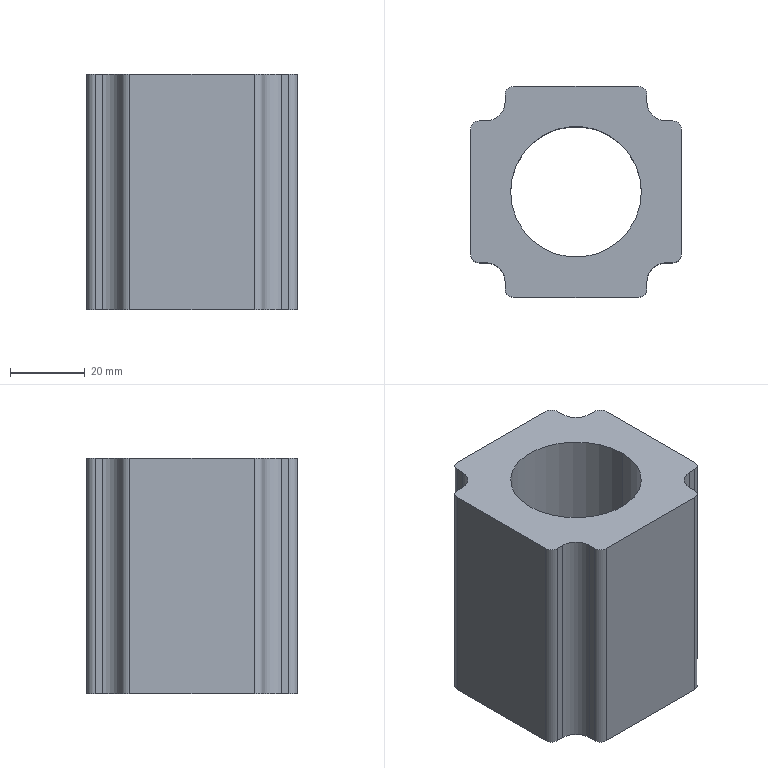Part | SolidWorks | features BaseBody 1 | 1 solid | 28 faces | box 56.4 x 56.4 x 63 mm | volume 119307 mm3 | cylinder 14 | plane 14 | commonest cylinder face diameters 4.6 x8 10 x4 34.98 x2
STEP:
#1=CARTESIAN_POINT('',(17.49,0.,-10.));
#2=VERTEX_POINT('',#1);
#3=CARTESIAN_POINT('',(-17.49,0.,-10.));
#4=VERTEX_POINT('',#3);
#5=CARTESIAN_POINT('',(0.,0.,-10.));
#6=DIRECTION('',(0.,0.,-1.));
#7=DIRECTION('',(-1.,0.,0.));
#8=AXIS2_PLACEMENT_3D('',#5,#6,#7);
#9=CIRCLE('',#8,17.49);
#10=EDGE_CURVE('',#2,#4,#9,.T.);
#11=ORIENTED_EDGE('',*,*,#10,.T.);
#12=CARTESIAN_POINT('',(-17.49,0.,53.));
#13=VERTEX_POINT('',#12);
#14=CARTESIAN_POINT('',(-17.49,0.,53.));
#15=DIRECTION('',(0.,0.,1.));
#16=VECTOR('',#15,1000.);
#17=LINE('',#14,#16);
#18=EDGE_CURVE('',#4,#13,#17,.T.);
#19=ORIENTED_EDGE('',*,*,#18,.T.);
#20=CARTESIAN_POINT('',(17.49,0.,53.));
#21=VERTEX_POINT('',#20);
#22=CARTESIAN_POINT('',(0.,0.,53.));
#23=DIRECTION('',(0.,0.,-1.));
#24=DIRECTION('',(1.,0.,0.));
#25=AXIS2_PLACEMENT_3D('',#22,#23,#24);
#26=CIRCLE('',#25,17.49);
#27=EDGE_CURVE('',#21,#13,#26,.T.);
#28=ORIENTED_EDGE('',*,*,#27,.F.);
#29=CARTESIAN_POINT('',(17.49,0.,53.));
#30=DIRECTION('',(0.,0.,1.));
#31=VECTOR('',#30,1000.);
#32=LINE('',#29,#31);
#33=EDGE_CURVE('',#2,#21,#32,.T.);
#34=ORIENTED_EDGE('',*,*,#33,.F.);
#35=EDGE_LOOP('',(#11,#19,#28,#34));
#36=FACE_OUTER_BOUND('',#35,.T.);
#37=CARTESIAN_POINT('',(0.,0.,53.));
#38=DIRECTION('',(0.,0.,1.));
#39=DIRECTION('',(1.,0.,0.));
#40=AXIS2_PLACEMENT_3D('',#37,#38,#39);
#41=CYLINDRICAL_SURFACE('',#40,17.49);
#42=ADVANCED_FACE('',(#36),#41,.F.);
#43=CARTESIAN_POINT('',(19.,-25.9,53.));
#44=VERTEX_POINT('',#43);
#45=CARTESIAN_POINT('',(19.,-24.,53.));
#46=VERTEX_POINT('',#45);
#47=CARTESIAN_POINT('',(19.,0.,53.));
#48=DIRECTION('',(0.,1.,0.));
#49=VECTOR('',#48,1000.);
#50=LINE('',#47,#49);
#51=EDGE_CURVE('',#44,#46,#50,.T.);
#52=ORIENTED_EDGE('',*,*,#51,.F.);
#53=CARTESIAN_POINT('',(19.,-25.9,-10.));
#54=VERTEX_POINT('',#53);
#55=CARTESIAN_POINT('',(19.,-25.9,122.091));
#56=DIRECTION('',(0.,0.,1.));
#57=VECTOR('',#56,1000.);
#58=LINE('',#55,#57);
#59=EDGE_CURVE('',#54,#44,#58,.T.);
#60=ORIENTED_EDGE('',*,*,#59,.F.);
#61=CARTESIAN_POINT('',(19.,-24.,-10.));
#62=VERTEX_POINT('',#61);
#63=CARTESIAN_POINT('',(19.,-24.,-10.));
#64=DIRECTION('',(0.,-1.,0.));
#65=VECTOR('',#64,1000.);
#66=LINE('',#63,#65);
#67=EDGE_CURVE('',#62,#54,#66,.T.);
#68=ORIENTED_EDGE('',*,*,#67,.F.);
#69=CARTESIAN_POINT('',(19.,-24.,-69.091));
#70=DIRECTION('',(0.,0.,1.));
#71=VECTOR('',#70,1000.);
#72=LINE('',#69,#71);
#73=EDGE_CURVE('',#62,#46,#72,.T.);
#74=ORIENTED_EDGE('',*,*,#73,.T.);
#75=EDGE_LOOP('',(#52,#60,#68,#74));
#76=FACE_OUTER_BOUND('',#75,.T.);
#77=CARTESIAN_POINT('',(19.,-28.2,0.));
#78=DIRECTION('',(1.,0.,0.));
#79=DIRECTION('',(0.,1.,0.));
#80=AXIS2_PLACEMENT_3D('',#77,#78,#79);
#81=PLANE('',#80);
#82=ADVANCED_FACE('',(#76),#81,.T.);
#83=ORIENTED_EDGE('',*,*,#73,.F.);
#84=CARTESIAN_POINT('',(24.,-19.,-10.));
#85=VERTEX_POINT('',#84);
#86=CARTESIAN_POINT('',(24.,-24.,-10.));
#87=DIRECTION('',(0.,0.,1.));
#88=DIRECTION('',(-1.,0.,0.));
#89=AXIS2_PLACEMENT_3D('',#86,#87,#88);
#90=CIRCLE('',#89,5.);
#91=EDGE_CURVE('',#85,#62,#90,.T.);
#92=ORIENTED_EDGE('',*,*,#91,.F.);
#93=CARTESIAN_POINT('',(24.,-19.,53.));
#94=VERTEX_POINT('',#93);
#95=CARTESIAN_POINT('',(24.,-19.,0.));
#96=DIRECTION('',(0.,0.,-1.));
#97=VECTOR('',#96,1000.);
#98=LINE('',#95,#97);
#99=EDGE_CURVE('',#94,#85,#98,.T.);
#100=ORIENTED_EDGE('',*,*,#99,.F.);
#101=CARTESIAN_POINT('',(24.,-24.,53.));
#102=DIRECTION('',(0.,0.,-1.));
#103=DIRECTION('',(1.,0.,0.));
#104=AXIS2_PLACEMENT_3D('',#101,#102,#103);
#105=CIRCLE('',#104,5.);
#106=EDGE_CURVE('',#46,#94,#105,.T.);
#107=ORIENTED_EDGE('',*,*,#106,.F.);
#108=EDGE_LOOP('',(#83,#92,#100,#107));
#109=FACE_OUTER_BOUND('',#108,.T.);
#110=CARTESIAN_POINT('',(24.,-24.,-69.091));
#111=DIRECTION('',(0.,0.,1.));
#112=DIRECTION('',(1.,0.,0.));
#113=AXIS2_PLACEMENT_3D('',#110,#111,#112);
#114=CYLINDRICAL_SURFACE('',#113,5.);
#115=ADVANCED_FACE('',(#109),#114,.F.);
#116=ORIENTED_EDGE('',*,*,#99,.T.);
#117=CARTESIAN_POINT('',(25.9,-19.,-10.));
#118=VERTEX_POINT('',#117);
#119=CARTESIAN_POINT('',(25.9,-19.,-10.));
#120=DIRECTION('',(-1.,0.,0.));
#121=VECTOR('',#120,1000.);
#122=LINE('',#119,#121);
#123=EDGE_CURVE('',#118,#85,#122,.T.);
#124=ORIENTED_EDGE('',*,*,#123,.F.);
#125=CARTESIAN_POINT('',(25.9,-19.,53.));
#126=VERTEX_POINT('',#125);
#127=CARTESIAN_POINT('',(25.9,-19.,122.091));
#128=DIRECTION('',(0.,0.,-1.));
#129=VECTOR('',#128,1000.);
#130=LINE('',#127,#129);
#131=EDGE_CURVE('',#126,#118,#130,.T.);
#132=ORIENTED_EDGE('',*,*,#131,.F.);
#133=CARTESIAN_POINT('',(0.,-19.,53.));
#134=DIRECTION('',(1.,0.,0.));
#135=VECTOR('',#134,1000.);
#136=LINE('',#133,#135);
#137=EDGE_CURVE('',#94,#126,#136,.T.);
#138=ORIENTED_EDGE('',*,*,#137,.F.);
#139=EDGE_LOOP('',(#116,#124,#132,#138));
#140=FACE_OUTER_BOUND('',#139,.T.);
#141=CARTESIAN_POINT('',(19.,-19.,0.));
#142=DIRECTION('',(0.,-1.,0.));
#143=DIRECTION('',(0.,0.,-1.));
#144=AXIS2_PLACEMENT_3D('',#141,#142,#143);
#145=PLANE('',#144);
#146=ADVANCED_FACE('',(#140),#145,.T.);
#147=ORIENTED_EDGE('',*,*,#131,.T.);
#148=CARTESIAN_POINT('',(28.2,-16.7,-10.));
#149=VERTEX_POINT('',#148);
#150=CARTESIAN_POINT('',(25.9,-16.7,-10.));
#151=DIRECTION('',(0.,0.,-1.));
#152=DIRECTION('',(-1.,0.,0.));
#153=AXIS2_PLACEMENT_3D('',#150,#151,#152);
#154=CIRCLE('',#153,2.3);
#155=EDGE_CURVE('',#149,#118,#154,.T.);
#156=ORIENTED_EDGE('',*,*,#155,.F.);
#157=CARTESIAN_POINT('',(28.2,-16.7,53.));
#158=VERTEX_POINT('',#157);
#159=CARTESIAN_POINT('',(28.2,-16.7,0.));
#160=DIRECTION('',(0.,0.,-1.));
#161=VECTOR('',#160,1000.);
#162=LINE('',#159,#161);
#163=EDGE_CURVE('',#158,#149,#162,.T.);
#164=ORIENTED_EDGE('',*,*,#163,.F.);
#165=CARTESIAN_POINT('',(25.9,-16.7,53.));
#166=DIRECTION('',(0.,0.,1.));
#167=DIRECTION('',(-1.,0.,0.));
#168=AXIS2_PLACEMENT_3D('',#165,#166,#167);
#169=CIRCLE('',#168,2.3);
#170=EDGE_CURVE('',#126,#158,#169,.T.);
#171=ORIENTED_EDGE('',*,*,#170,.F.);
#172=EDGE_LOOP('',(#147,#156,#164,#171));
#173=FACE_OUTER_BOUND('',#172,.T.);
#174=CARTESIAN_POINT('',(25.9,-16.7,122.091));
#175=DIRECTION('',(0.,0.,-1.));
#176=DIRECTION('',(-1.,0.,0.));
#177=AXIS2_PLACEMENT_3D('',#174,#175,#176);
#178=CYLINDRICAL_SURFACE('',#177,2.3);
#179=ADVANCED_FACE('',(#173),#178,.T.);
#180=CARTESIAN_POINT('',(28.2,16.7,53.));
#181=VERTEX_POINT('',#180);
#182=CARTESIAN_POINT('',(28.2,0.,53.));
#183=DIRECTION('',(0.,1.,0.));
#184=VECTOR('',#183,1000.);
#185=LINE('',#182,#184);
#186=EDGE_CURVE('',#158,#181,#185,.T.);
#187=ORIENTED_EDGE('',*,*,#186,.F.);
#188=ORIENTED_EDGE('',*,*,#163,.T.);
#189=CARTESIAN_POINT('',(28.2,16.7,-10.));
#190=VERTEX_POINT('',#189);
#191=CARTESIAN_POINT('',(28.2,16.7,-10.));
#192=DIRECTION('',(0.,-1.,0.));
#193=VECTOR('',#192,1000.);
#194=LINE('',#191,#193);
#195=EDGE_CURVE('',#190,#149,#194,.T.);
#196=ORIENTED_EDGE('',*,*,#195,.F.);
#197=CARTESIAN_POINT('',(28.2,16.7,122.091));
#198=DIRECTION('',(0.,0.,-1.));
#199=VECTOR('',#198,1000.);
#200=LINE('',#197,#199);
#201=EDGE_CURVE('',#181,#190,#200,.T.);
#202=ORIENTED_EDGE('',*,*,#201,.F.);
#203=EDGE_LOOP('',(#187,#188,#196,#202));
#204=FACE_OUTER_BOUND('',#203,.T.);
#205=CARTESIAN_POINT('',(28.2,-19.,0.));
#206=DIRECTION('',(1.,0.,0.));
#207=DIRECTION('',(0.,1.,0.));
#208=AXIS2_PLACEMENT_3D('',#205,#206,#207);
#209=PLANE('',#208);
#210=ADVANCED_FACE('',(#204),#209,.T.);
#211=ORIENTED_EDGE('',*,*,#201,.T.);
#212=CARTESIAN_POINT('',(25.9,19.,-10.));
#213=VERTEX_POINT('',#212);
#214=CARTESIAN_POINT('',(25.9,16.7,-10.));
#215=DIRECTION('',(0.,0.,-1.));
#216=DIRECTION('',(-1.,0.,0.));
#217=AXIS2_PLACEMENT_3D('',#214,#215,#216);
#218=CIRCLE('',#217,2.3);
#219=EDGE_CURVE('',#213,#190,#218,.T.);
#220=ORIENTED_EDGE('',*,*,#219,.F.);
#221=CARTESIAN_POINT('',(25.9,19.,53.));
#222=VERTEX_POINT('',#221);
#223=CARTESIAN_POINT('',(25.9,19.,0.));
#224=DIRECTION('',(0.,0.,-1.));
#225=VECTOR('',#224,1000.);
#226=LINE('',#223,#225);
#227=EDGE_CURVE('',#222,#213,#226,.T.);
#228=ORIENTED_EDGE('',*,*,#227,.F.);
#229=CARTESIAN_POINT('',(25.9,16.7,53.));
#230=DIRECTION('',(0.,0.,1.));
#231=DIRECTION('',(-1.,0.,0.));
#232=AXIS2_PLACEMENT_3D('',#229,#230,#231);
#233=CIRCLE('',#232,2.3);
#234=EDGE_CURVE('',#181,#222,#233,.T.);
#235=ORIENTED_EDGE('',*,*,#234,.F.);
#236=EDGE_LOOP('',(#211,#220,#228,#235));
#237=FACE_OUTER_BOUND('',#236,.T.);
#238=CARTESIAN_POINT('',(25.9,16.7,122.091));
#239=DIRECTION('',(0.,0.,-1.));
#240=DIRECTION('',(-1.,0.,0.));
#241=AXIS2_PLACEMENT_3D('',#238,#239,#240);
#242=CYLINDRICAL_SURFACE('',#241,2.3);
#243=ADVANCED_FACE('',(#237),#242,.T.);
#244=CARTESIAN_POINT('',(24.,19.,53.));
#245=VERTEX_POINT('',#244);
#246=CARTESIAN_POINT('',(0.,19.,53.));
#247=DIRECTION('',(-1.,0.,0.));
#248=VECTOR('',#247,1000.);
#249=LINE('',#246,#248);
#250=EDGE_CURVE('',#222,#245,#249,.T.);
#251=ORIENTED_EDGE('',*,*,#250,.F.);
#252=ORIENTED_EDGE('',*,*,#227,.T.);
#253=CARTESIAN_POINT('',(24.,19.,-10.));
#254=VERTEX_POINT('',#253);
#255=CARTESIAN_POINT('',(24.,19.,-10.));
#256=DIRECTION('',(1.,0.,0.));
#257=VECTOR('',#256,1000.);
#258=LINE('',#255,#257);
#259=EDGE_CURVE('',#254,#213,#258,.T.);
#260=ORIENTED_EDGE('',*,*,#259,.F.);
#261=CARTESIAN_POINT('',(24.,19.,-69.091));
#262=DIRECTION('',(0.,0.,1.));
#263=VECTOR('',#262,1000.);
#264=LINE('',#261,#263);
#265=EDGE_CURVE('',#254,#245,#264,.T.);
#266=ORIENTED_EDGE('',*,*,#265,.T.);
#267=EDGE_LOOP('',(#251,#252,#260,#266));
#268=FACE_OUTER_BOUND('',#267,.T.);
#269=CARTESIAN_POINT('',(28.2,19.,0.));
#270=DIRECTION('',(0.,1.,0.));
#271=DIRECTION('',(1.,0.,0.));
#272=AXIS2_PLACEMENT_3D('',#269,#270,#271);
#273=PLANE('',#272);
#274=ADVANCED_FACE('',(#268),#273,.T.);
#275=ORIENTED_EDGE('',*,*,#265,.F.);
#276=CARTESIAN_POINT('',(19.,24.,-10.));
#277=VERTEX_POINT('',#276);
#278=CARTESIAN_POINT('',(24.,24.,-10.));
#279=DIRECTION('',(0.,0.,1.));
#280=DIRECTION('',(-1.,0.,0.));
#281=AXIS2_PLACEMENT_3D('',#278,#279,#280);
#282=CIRCLE('',#281,5.);
#283=EDGE_CURVE('',#277,#254,#282,.T.);
#284=ORIENTED_EDGE('',*,*,#283,.F.);
#285=CARTESIAN_POINT('',(19.,24.,53.));
#286=VERTEX_POINT('',#285);
#287=CARTESIAN_POINT('',(19.,24.,0.));
#288=DIRECTION('',(0.,0.,-1.));
#289=VECTOR('',#288,1000.);
#290=LINE('',#287,#289);
#291=EDGE_CURVE('',#286,#277,#290,.T.);
#292=ORIENTED_EDGE('',*,*,#291,.F.);
#293=CARTESIAN_POINT('',(24.,24.,53.));
#294=DIRECTION('',(0.,0.,-1.));
#295=DIRECTION('',(1.,0.,0.));
#296=AXIS2_PLACEMENT_3D('',#293,#294,#295);
#297=CIRCLE('',#296,5.);
#298=EDGE_CURVE('',#245,#286,#297,.T.);
#299=ORIENTED_EDGE('',*,*,#298,.F.);
#300=EDGE_LOOP('',(#275,#284,#292,#299));
#301=FACE_OUTER_BOUND('',#300,.T.);
#302=CARTESIAN_POINT('',(24.,24.,-69.091));
#303=DIRECTION('',(0.,0.,1.));
#304=DIRECTION('',(1.,0.,0.));
#305=AXIS2_PLACEMENT_3D('',#302,#303,#304);
#306=CYLINDRICAL_SURFACE('',#305,5.);
#307=ADVANCED_FACE('',(#301),#306,.F.);
#308=ORIENTED_EDGE('',*,*,#291,.T.);
#309=CARTESIAN_POINT('',(19.,25.9,-10.));
#310=VERTEX_POINT('',#309);
#311=CARTESIAN_POINT('',(19.,25.9,-10.));
#312=DIRECTION('',(0.,-1.,0.));
#313=VECTOR('',#312,1000.);
#314=LINE('',#311,#313);
#315=EDGE_CURVE('',#310,#277,#314,.T.);
#316=ORIENTED_EDGE('',*,*,#315,.F.);
#317=CARTESIAN_POINT('',(19.,25.9,53.));
#318=VERTEX_POINT('',#317);
#319=CARTESIAN_POINT('',(19.,25.9,122.091));
#320=DIRECTION('',(0.,0.,-1.));
#321=VECTOR('',#320,1000.);
#322=LINE('',#319,#321);
#323=EDGE_CURVE('',#318,#310,#322,.T.);
#324=ORIENTED_EDGE('',*,*,#323,.F.);
#325=CARTESIAN_POINT('',(19.,0.,53.));
#326=DIRECTION('',(0.,1.,0.));
#327=VECTOR('',#326,1000.);
#328=LINE('',#325,#327);
#329=EDGE_CURVE('',#286,#318,#328,.T.);
#330=ORIENTED_EDGE('',*,*,#329,.F.);
#331=EDGE_LOOP('',(#308,#316,#324,#330));
#332=FACE_OUTER_BOUND('',#331,.T.);
#333=CARTESIAN_POINT('',(19.,19.,0.));
#334=DIRECTION('',(1.,0.,0.));
#335=DIRECTION('',(0.,1.,0.));
#336=AXIS2_PLACEMENT_3D('',#333,#334,#335);
#337=PLANE('',#336);
#338=ADVANCED_FACE('',(#332),#337,.T.);
#339=ORIENTED_EDGE('',*,*,#323,.T.);
#340=CARTESIAN_POINT('',(16.7,28.2,-10.));
#341=VERTEX_POINT('',#340);
#342=CARTESIAN_POINT('',(16.7,25.9,-10.));
#343=DIRECTION('',(0.,0.,-1.));
#344=DIRECTION('',(-1.,0.,0.));
#345=AXIS2_PLACEMENT_3D('',#342,#343,#344);
#346=CIRCLE('',#345,2.3);
#347=EDGE_CURVE('',#341,#310,#346,.T.);
#348=ORIENTED_EDGE('',*,*,#347,.F.);
#349=CARTESIAN_POINT('',(16.7,28.2,53.));
#350=VERTEX_POINT('',#349);
#351=CARTESIAN_POINT('',(16.7,28.2,0.));
#352=DIRECTION('',(0.,0.,-1.));
#353=VECTOR('',#352,1000.);
#354=LINE('',#351,#353);
#355=EDGE_CURVE('',#350,#341,#354,.T.);
#356=ORIENTED_EDGE('',*,*,#355,.F.);
#357=CARTESIAN_POINT('',(16.7,25.9,53.));
#358=DIRECTION('',(0.,0.,1.));
#359=DIRECTION('',(-1.,0.,0.));
#360=AXIS2_PLACEMENT_3D('',#357,#358,#359);
#361=CIRCLE('',#360,2.3);
#362=EDGE_CURVE('',#318,#350,#361,.T.);
#363=ORIENTED_EDGE('',*,*,#362,.F.);
#364=EDGE_LOOP('',(#339,#348,#356,#363));
#365=FACE_OUTER_BOUND('',#364,.T.);
#366=CARTESIAN_POINT('',(16.7,25.9,122.091));
#367=DIRECTION('',(0.,0.,-1.));
#368=DIRECTION('',(-1.,0.,0.));
#369=AXIS2_PLACEMENT_3D('',#366,#367,#368);
#370=CYLINDRICAL_SURFACE('',#369,2.3);
#371=ADVANCED_FACE('',(#365),#370,.T.);
#372=CARTESIAN_POINT('',(-16.7,28.2,53.));
#373=VERTEX_POINT('',#372);
#374=CARTESIAN_POINT('',(0.,28.2,53.));
#375=DIRECTION('',(-1.,0.,0.));
#376=VECTOR('',#375,1000.);
#377=LINE('',#374,#376);
#378=EDGE_CURVE('',#350,#373,#377,.T.);
#379=ORIENTED_EDGE('',*,*,#378,.F.);
#380=ORIENTED_EDGE('',*,*,#355,.T.);
#381=CARTESIAN_POINT('',(-16.7,28.2,-10.));
#382=VERTEX_POINT('',#381);
#383=CARTESIAN_POINT('',(-16.7,28.2,-10.));
#384=DIRECTION('',(1.,0.,0.));
#385=VECTOR('',#384,1000.);
#386=LINE('',#383,#385);
#387=EDGE_CURVE('',#382,#341,#386,.T.);
#388=ORIENTED_EDGE('',*,*,#387,.F.);
#389=CARTESIAN_POINT('',(-16.7,28.2,122.091));
#390=DIRECTION('',(0.,0.,-1.));
#391=VECTOR('',#390,1000.);
#392=LINE('',#389,#391);
#393=EDGE_CURVE('',#373,#382,#392,.T.);
#394=ORIENTED_EDGE('',*,*,#393,.F.);
#395=EDGE_LOOP('',(#379,#380,#388,#394));
#396=FACE_OUTER_BOUND('',#395,.T.);
#397=CARTESIAN_POINT('',(19.,28.2,0.));
#398=DIRECTION('',(0.,1.,0.));
#399=DIRECTION('',(1.,0.,0.));
#400=AXIS2_PLACEMENT_3D('',#397,#398,#399);
#401=PLANE('',#400);
#402=ADVANCED_FACE('',(#396),#401,.T.);
#403=ORIENTED_EDGE('',*,*,#393,.T.);
#404=CARTESIAN_POINT('',(-19.,25.9,-10.));
#405=VERTEX_POINT('',#404);
#406=CARTESIAN_POINT('',(-16.7,25.9,-10.));
#407=DIRECTION('',(0.,0.,-1.));
#408=DIRECTION('',(-1.,0.,0.));
#409=AXIS2_PLACEMENT_3D('',#406,#407,#408);
#410=CIRCLE('',#409,2.3);
#411=EDGE_CURVE('',#405,#382,#410,.T.);
#412=ORIENTED_EDGE('',*,*,#411,.F.);
#413=CARTESIAN_POINT('',(-19.,25.9,53.));
#414=VERTEX_POINT('',#413);
#415=CARTESIAN_POINT('',(-19.,25.9,0.));
#416=DIRECTION('',(0.,0.,-1.));
#417=VECTOR('',#416,1000.);
#418=LINE('',#415,#417);
#419=EDGE_CURVE('',#414,#405,#418,.T.);
#420=ORIENTED_EDGE('',*,*,#419,.F.);
#421=CARTESIAN_POINT('',(-16.7,25.9,53.));
#422=DIRECTION('',(0.,0.,1.));
#423=DIRECTION('',(-1.,0.,0.));
#424=AXIS2_PLACEMENT_3D('',#421,#422,#423);
#425=CIRCLE('',#424,2.3);
#426=EDGE_CURVE('',#373,#414,#425,.T.);
#427=ORIENTED_EDGE('',*,*,#426,.F.);
#428=EDGE_LOOP('',(#403,#412,#420,#427));
#429=FACE_OUTER_BOUND('',#428,.T.);
#430=CARTESIAN_POINT('',(-16.7,25.9,122.091));
#431=DIRECTION('',(0.,0.,-1.));
#432=DIRECTION('',(-1.,0.,0.));
#433=AXIS2_PLACEMENT_3D('',#430,#431,#432);
#434=CYLINDRICAL_SURFACE('',#433,2.3);
#435=ADVANCED_FACE('',(#429),#434,.T.);
#436=CARTESIAN_POINT('',(-19.,24.,53.));
#437=VERTEX_POINT('',#436);
#438=CARTESIAN_POINT('',(-19.,0.,53.));
#439=DIRECTION('',(0.,-1.,0.));
#440=VECTOR('',#439,1000.);
#441=LINE('',#438,#440);
#442=EDGE_CURVE('',#414,#437,#441,.T.);
#443=ORIENTED_EDGE('',*,*,#442,.F.);
#444=ORIENTED_EDGE('',*,*,#419,.T.);
#445=CARTESIAN_POINT('',(-19.,24.,-10.));
#446=VERTEX_POINT('',#445);
#447=CARTESIAN_POINT('',(-19.,24.,-10.));
#448=DIRECTION('',(0.,1.,0.));
#449=VECTOR('',#448,1000.);
#450=LINE('',#447,#449);
#451=EDGE_CURVE('',#446,#405,#450,.T.);
#452=ORIENTED_EDGE('',*,*,#451,.F.);
#453=CARTESIAN_POINT('',(-19.,24.,-69.091));
#454=DIRECTION('',(0.,0.,1.));
#455=VECTOR('',#454,1000.);
#456=LINE('',#453,#455);
#457=EDGE_CURVE('',#446,#437,#456,.T.);
#458=ORIENTED_EDGE('',*,*,#457,.T.);
#459=EDGE_LOOP('',(#443,#444,#452,#458));
#460=FACE_OUTER_BOUND('',#459,.T.);
#461=CARTESIAN_POINT('',(-19.,28.2,0.));
#462=DIRECTION('',(-1.,0.,0.));
#463=DIRECTION('',(0.,0.,1.));
#464=AXIS2_PLACEMENT_3D('',#461,#462,#463);
#465=PLANE('',#464);
#466=ADVANCED_FACE('',(#460),#465,.T.);
#467=ORIENTED_EDGE('',*,*,#457,.F.);
#468=CARTESIAN_POINT('',(-24.,19.,-10.));
#469=VERTEX_POINT('',#468);
#470=CARTESIAN_POINT('',(-24.,24.,-10.));
#471=DIRECTION('',(0.,0.,1.));
#472=DIRECTION('',(-1.,0.,0.));
#473=AXIS2_PLACEMENT_3D('',#470,#471,#472);
#474=CIRCLE('',#473,5.);
#475=EDGE_CURVE('',#469,#446,#474,.T.);
#476=ORIENTED_EDGE('',*,*,#475,.F.);
#477=CARTESIAN_POINT('',(-24.,19.,53.));
#478=VERTEX_POINT('',#477);
#479=CARTESIAN_POINT('',(-24.,19.,0.));
#480=DIRECTION('',(0.,0.,-1.));
#481=VECTOR('',#480,1000.);
#482=LINE('',#479,#481);
#483=EDGE_CURVE('',#478,#469,#482,.T.);
#484=ORIENTED_EDGE('',*,*,#483,.F.);
#485=CARTESIAN_POINT('',(-24.,24.,53.));
#486=DIRECTION('',(0.,0.,-1.));
#487=DIRECTION('',(1.,0.,0.));
#488=AXIS2_PLACEMENT_3D('',#485,#486,#487);
#489=CIRCLE('',#488,5.);
#490=EDGE_CURVE('',#437,#478,#489,.T.);
#491=ORIENTED_EDGE('',*,*,#490,.F.);
#492=EDGE_LOOP('',(#467,#476,#484,#491));
#493=FACE_OUTER_BOUND('',#492,.T.);
#494=CARTESIAN_POINT('',(-24.,24.,-69.091));
#495=DIRECTION('',(0.,0.,1.));
#496=DIRECTION('',(1.,0.,0.));
#497=AXIS2_PLACEMENT_3D('',#494,#495,#496);
#498=CYLINDRICAL_SURFACE('',#497,5.);
#499=ADVANCED_FACE('',(#493),#498,.F.);
#500=ORIENTED_EDGE('',*,*,#483,.T.);
#501=CARTESIAN_POINT('',(-25.9,19.,-10.));
#502=VERTEX_POINT('',#501);
#503=CARTESIAN_POINT('',(-25.9,19.,-10.));
#504=DIRECTION('',(1.,0.,0.));
#505=VECTOR('',#504,1000.);
#506=LINE('',#503,#505);
#507=EDGE_CURVE('',#502,#469,#506,.T.);
#508=ORIENTED_EDGE('',*,*,#507,.F.);
#509=CARTESIAN_POINT('',(-25.9,19.,53.));
#510=VERTEX_POINT('',#509);
#511=CARTESIAN_POINT('',(-25.9,19.,122.091));
#512=DIRECTION('',(0.,0.,-1.));
#513=VECTOR('',#512,1000.);
#514=LINE('',#511,#513);
#515=EDGE_CURVE('',#510,#502,#514,.T.);
#516=ORIENTED_EDGE('',*,*,#515,.F.);
#517=CARTESIAN_POINT('',(0.,19.,53.));
#518=DIRECTION('',(-1.,0.,0.));
#519=VECTOR('',#518,1000.);
#520=LINE('',#517,#519);
#521=EDGE_CURVE('',#478,#510,#520,.T.);
#522=ORIENTED_EDGE('',*,*,#521,.F.);
#523=EDGE_LOOP('',(#500,#508,#516,#522));
#524=FACE_OUTER_BOUND('',#523,.T.);
#525=CARTESIAN_POINT('',(-19.,19.,0.));
#526=DIRECTION('',(0.,1.,0.));
#527=DIRECTION('',(1.,0.,0.));
#528=AXIS2_PLACEMENT_3D('',#525,#526,#527);
#529=PLANE('',#528);
#530=ADVANCED_FACE('',(#524),#529,.T.);
#531=ORIENTED_EDGE('',*,*,#515,.T.);
#532=CARTESIAN_POINT('',(-28.2,16.7,-10.));
#533=VERTEX_POINT('',#532);
#534=CARTESIAN_POINT('',(-25.9,16.7,-10.));
#535=DIRECTION('',(0.,0.,-1.));
#536=DIRECTION('',(-1.,0.,0.));
#537=AXIS2_PLACEMENT_3D('',#534,#535,#536);
#538=CIRCLE('',#537,2.3);
#539=EDGE_CURVE('',#533,#502,#538,.T.);
#540=ORIENTED_EDGE('',*,*,#539,.F.);
#541=CARTESIAN_POINT('',(-28.2,16.7,53.));
#542=VERTEX_POINT('',#541);
#543=CARTESIAN_POINT('',(-28.2,16.7,0.));
#544=DIRECTION('',(0.,0.,-1.));
#545=VECTOR('',#544,1000.);
#546=LINE('',#543,#545);
#547=EDGE_CURVE('',#542,#533,#546,.T.);
#548=ORIENTED_EDGE('',*,*,#547,.F.);
#549=CARTESIAN_POINT('',(-25.9,16.7,53.));
#550=DIRECTION('',(0.,0.,1.));
#551=DIRECTION('',(-1.,0.,0.));
#552=AXIS2_PLACEMENT_3D('',#549,#550,#551);
#553=CIRCLE('',#552,2.3);
#554=EDGE_CURVE('',#510,#542,#553,.T.);
#555=ORIENTED_EDGE('',*,*,#554,.F.);
#556=EDGE_LOOP('',(#531,#540,#548,#555));
#557=FACE_OUTER_BOUND('',#556,.T.);
#558=CARTESIAN_POINT('',(-25.9,16.7,122.091));
#559=DIRECTION('',(0.,0.,-1.));
#560=DIRECTION('',(-1.,0.,0.));
#561=AXIS2_PLACEMENT_3D('',#558,#559,#560);
#562=CYLINDRICAL_SURFACE('',#561,2.3);
#563=ADVANCED_FACE('',(#557),#562,.T.);
#564=CARTESIAN_POINT('',(-28.2,-16.7,53.));
#565=VERTEX_POINT('',#564);
#566=CARTESIAN_POINT('',(-28.2,0.,53.));
#567=DIRECTION('',(0.,-1.,0.));
#568=VECTOR('',#567,1000.);
#569=LINE('',#566,#568);
#570=EDGE_CURVE('',#542,#565,#569,.T.);
#571=ORIENTED_EDGE('',*,*,#570,.F.);
#572=ORIENTED_EDGE('',*,*,#547,.T.);
#573=CARTESIAN_POINT('',(-28.2,-16.7,-10.));
#574=VERTEX_POINT('',#573);
#575=CARTESIAN_POINT('',(-28.2,-16.7,-10.));
#576=DIRECTION('',(0.,1.,0.));
#577=VECTOR('',#576,1000.);
#578=LINE('',#575,#577);
#579=EDGE_CURVE('',#574,#533,#578,.T.);
#580=ORIENTED_EDGE('',*,*,#579,.F.);
#581=CARTESIAN_POINT('',(-28.2,-16.7,122.091));
#582=DIRECTION('',(0.,0.,-1.));
#583=VECTOR('',#582,1000.);
#584=LINE('',#581,#583);
#585=EDGE_CURVE('',#565,#574,#584,.T.);
#586=ORIENTED_EDGE('',*,*,#585,.F.);
#587=EDGE_LOOP('',(#571,#572,#580,#586));
#588=FACE_OUTER_BOUND('',#587,.T.);
#589=CARTESIAN_POINT('',(-28.2,19.,0.));
#590=DIRECTION('',(-1.,0.,0.));
#591=DIRECTION('',(0.,0.,1.));
#592=AXIS2_PLACEMENT_3D('',#589,#590,#591);
#593=PLANE('',#592);
#594=ADVANCED_FACE('',(#588),#593,.T.);
#595=ORIENTED_EDGE('',*,*,#585,.T.);
#596=CARTESIAN_POINT('',(-25.9,-19.,-10.));
#597=VERTEX_POINT('',#596);
#598=CARTESIAN_POINT('',(-25.9,-16.7,-10.));
#599=DIRECTION('',(0.,0.,-1.));
#600=DIRECTION('',(-1.,0.,0.));
#601=AXIS2_PLACEMENT_3D('',#598,#599,#600);
#602=CIRCLE('',#601,2.3);
#603=EDGE_CURVE('',#597,#574,#602,.T.);
#604=ORIENTED_EDGE('',*,*,#603,.F.);
#605=CARTESIAN_POINT('',(-25.9,-19.,53.));
#606=VERTEX_POINT('',#605);
#607=CARTESIAN_POINT('',(-25.9,-19.,0.));
#608=DIRECTION('',(0.,0.,-1.));
#609=VECTOR('',#608,1000.);
#610=LINE('',#607,#609);
#611=EDGE_CURVE('',#606,#597,#610,.T.);
#612=ORIENTED_EDGE('',*,*,#611,.F.);
#613=CARTESIAN_POINT('',(-25.9,-16.7,53.));
#614=DIRECTION('',(0.,0.,1.));
#615=DIRECTION('',(-1.,0.,0.));
#616=AXIS2_PLACEMENT_3D('',#613,#614,#615);
#617=CIRCLE('',#616,2.3);
#618=EDGE_CURVE('',#565,#606,#617,.T.);
#619=ORIENTED_EDGE('',*,*,#618,.F.);
#620=EDGE_LOOP('',(#595,#604,#612,#619));
#621=FACE_OUTER_BOUND('',#620,.T.);
#622=CARTESIAN_POINT('',(-25.9,-16.7,122.091));
#623=DIRECTION('',(0.,0.,-1.));
#624=DIRECTION('',(-1.,0.,0.));
#625=AXIS2_PLACEMENT_3D('',#622,#623,#624);
#626=CYLINDRICAL_SURFACE('',#625,2.3);
#627=ADVANCED_FACE('',(#621),#626,.T.);
#628=CARTESIAN_POINT('',(-24.,-19.,53.));
#629=VERTEX_POINT('',#628);
#630=CARTESIAN_POINT('',(0.,-19.,53.));
#631=DIRECTION('',(1.,0.,0.));
#632=VECTOR('',#631,1000.);
#633=LINE('',#630,#632);
#634=EDGE_CURVE('',#606,#629,#633,.T.);
#635=ORIENTED_EDGE('',*,*,#634,.F.);
#636=ORIENTED_EDGE('',*,*,#611,.T.);
#637=CARTESIAN_POINT('',(-24.,-19.,-10.));
#638=VERTEX_POINT('',#637);
#639=CARTESIAN_POINT('',(-24.,-19.,-10.));
#640=DIRECTION('',(-1.,0.,0.));
#641=VECTOR('',#640,1000.);
#642=LINE('',#639,#641);
#643=EDGE_CURVE('',#638,#597,#642,.T.);
#644=ORIENTED_EDGE('',*,*,#643,.F.);
#645=CARTESIAN_POINT('',(-24.,-19.,-69.091));
#646=DIRECTION('',(0.,0.,1.));
#647=VECTOR('',#646,1000.);
#648=LINE('',#645,#647);
#649=EDGE_CURVE('',#638,#629,#648,.T.);
#650=ORIENTED_EDGE('',*,*,#649,.T.);
#651=EDGE_LOOP('',(#635,#636,#644,#650));
#652=FACE_OUTER_BOUND('',#651,.T.);
#653=CARTESIAN_POINT('',(-28.2,-19.,0.));
#654=DIRECTION('',(0.,-1.,0.));
#655=DIRECTION('',(0.,0.,-1.));
#656=AXIS2_PLACEMENT_3D('',#653,#654,#655);
#657=PLANE('',#656);
#658=ADVANCED_FACE('',(#652),#657,.T.);
#659=ORIENTED_EDGE('',*,*,#649,.F.);
#660=CARTESIAN_POINT('',(-19.,-24.,-10.));
#661=VERTEX_POINT('',#660);
#662=CARTESIAN_POINT('',(-24.,-24.,-10.));
#663=DIRECTION('',(0.,0.,1.));
#664=DIRECTION('',(-1.,0.,0.));
#665=AXIS2_PLACEMENT_3D('',#662,#663,#664);
#666=CIRCLE('',#665,5.);
#667=EDGE_CURVE('',#661,#638,#666,.T.);
#668=ORIENTED_EDGE('',*,*,#667,.F.);
#669=CARTESIAN_POINT('',(-19.,-24.,53.));
#670=VERTEX_POINT('',#669);
#671=CARTESIAN_POINT('',(-19.,-24.,0.));
#672=DIRECTION('',(0.,0.,-1.));
#673=VECTOR('',#672,1000.);
#674=LINE('',#671,#673);
#675=EDGE_CURVE('',#670,#661,#674,.T.);
#676=ORIENTED_EDGE('',*,*,#675,.F.);
#677=CARTESIAN_POINT('',(-24.,-24.,53.));
#678=DIRECTION('',(0.,0.,-1.));
#679=DIRECTION('',(1.,0.,0.));
#680=AXIS2_PLACEMENT_3D('',#677,#678,#679);
#681=CIRCLE('',#680,5.);
#682=EDGE_CURVE('',#629,#670,#681,.T.);
#683=ORIENTED_EDGE('',*,*,#682,.F.);
#684=EDGE_LOOP('',(#659,#668,#676,#683));
#685=FACE_OUTER_BOUND('',#684,.T.);
#686=CARTESIAN_POINT('',(-24.,-24.,-69.091));
#687=DIRECTION('',(0.,0.,1.));
#688=DIRECTION('',(1.,0.,0.));
#689=AXIS2_PLACEMENT_3D('',#686,#687,#688);
#690=CYLINDRICAL_SURFACE('',#689,5.);
#691=ADVANCED_FACE('',(#685),#690,.F.);
#692=ORIENTED_EDGE('',*,*,#675,.T.);
#693=CARTESIAN_POINT('',(-19.,-25.9,-10.));
#694=VERTEX_POINT('',#693);
#695=CARTESIAN_POINT('',(-19.,-25.9,-10.));
#696=DIRECTION('',(0.,1.,0.));
#697=VECTOR('',#696,1000.);
#698=LINE('',#695,#697);
#699=EDGE_CURVE('',#694,#661,#698,.T.);
#700=ORIENTED_EDGE('',*,*,#699,.F.);
#701=CARTESIAN_POINT('',(-19.,-25.9,53.));
#702=VERTEX_POINT('',#701);
#703=CARTESIAN_POINT('',(-19.,-25.9,122.091));
#704=DIRECTION('',(0.,0.,-1.));
#705=VECTOR('',#704,1000.);
#706=LINE('',#703,#705);
#707=EDGE_CURVE('',#702,#694,#706,.T.);
#708=ORIENTED_EDGE('',*,*,#707,.F.);
#709=CARTESIAN_POINT('',(-19.,0.,53.));
#710=DIRECTION('',(0.,-1.,0.));
#711=VECTOR('',#710,1000.);
#712=LINE('',#709,#711);
#713=EDGE_CURVE('',#670,#702,#712,.T.);
#714=ORIENTED_EDGE('',*,*,#713,.F.);
#715=EDGE_LOOP('',(#692,#700,#708,#714));
#716=FACE_OUTER_BOUND('',#715,.T.);
#717=CARTESIAN_POINT('',(-19.,-19.,0.));
#718=DIRECTION('',(-1.,0.,0.));
#719=DIRECTION('',(0.,0.,1.));
#720=AXIS2_PLACEMENT_3D('',#717,#718,#719);
#721=PLANE('',#720);
#722=ADVANCED_FACE('',(#716),#721,.T.);
#723=ORIENTED_EDGE('',*,*,#707,.T.);
#724=CARTESIAN_POINT('',(-16.7,-28.2,-10.));
#725=VERTEX_POINT('',#724);
#726=CARTESIAN_POINT('',(-16.7,-25.9,-10.));
#727=DIRECTION('',(0.,0.,-1.));
#728=DIRECTION('',(-1.,0.,0.));
#729=AXIS2_PLACEMENT_3D('',#726,#727,#728);
#730=CIRCLE('',#729,2.3);
#731=EDGE_CURVE('',#725,#694,#730,.T.);
#732=ORIENTED_EDGE('',*,*,#731,.F.);
#733=CARTESIAN_POINT('',(-16.7,-28.2,53.));
#734=VERTEX_POINT('',#733);
#735=CARTESIAN_POINT('',(-16.7,-28.2,0.));
#736=DIRECTION('',(0.,0.,-1.));
#737=VECTOR('',#736,1000.);
#738=LINE('',#735,#737);
#739=EDGE_CURVE('',#734,#725,#738,.T.);
#740=ORIENTED_EDGE('',*,*,#739,.F.);
#741=CARTESIAN_POINT('',(-16.7,-25.9,53.));
#742=DIRECTION('',(0.,0.,1.));
#743=DIRECTION('',(-1.,0.,0.));
#744=AXIS2_PLACEMENT_3D('',#741,#742,#743);
#745=CIRCLE('',#744,2.3);
#746=EDGE_CURVE('',#702,#734,#745,.T.);
#747=ORIENTED_EDGE('',*,*,#746,.F.);
#748=EDGE_LOOP('',(#723,#732,#740,#747));
#749=FACE_OUTER_BOUND('',#748,.T.);
#750=CARTESIAN_POINT('',(-16.7,-25.9,122.091));
#751=DIRECTION('',(0.,0.,-1.));
#752=DIRECTION('',(-1.,0.,0.));
#753=AXIS2_PLACEMENT_3D('',#750,#751,#752);
#754=CYLINDRICAL_SURFACE('',#753,2.3);
#755=ADVANCED_FACE('',(#749),#754,.T.);
#756=ORIENTED_EDGE('',*,*,#739,.T.);
#757=CARTESIAN_POINT('',(16.7,-28.2,-10.));
#758=VERTEX_POINT('',#757);
#759=CARTESIAN_POINT('',(16.7,-28.2,-10.));
#760=DIRECTION('',(-1.,0.,0.));
#761=VECTOR('',#760,1000.);
#762=LINE('',#759,#761);
#763=EDGE_CURVE('',#758,#725,#762,.T.);
#764=ORIENTED_EDGE('',*,*,#763,.F.);
#765=CARTESIAN_POINT('',(16.7,-28.2,53.));
#766=VERTEX_POINT('',#765);
#767=CARTESIAN_POINT('',(16.7,-28.2,122.091));
#768=DIRECTION('',(0.,0.,-1.));
#769=VECTOR('',#768,1000.);
#770=LINE('',#767,#769);
#771=EDGE_CURVE('',#766,#758,#770,.T.);
#772=ORIENTED_EDGE('',*,*,#771,.F.);
#773=CARTESIAN_POINT('',(0.,-28.2,53.));
#774=DIRECTION('',(1.,0.,0.));
#775=VECTOR('',#774,1000.);
#776=LINE('',#773,#775);
#777=EDGE_CURVE('',#734,#766,#776,.T.);
#778=ORIENTED_EDGE('',*,*,#777,.F.);
#779=EDGE_LOOP('',(#756,#764,#772,#778));
#780=FACE_OUTER_BOUND('',#779,.T.);
#781=CARTESIAN_POINT('',(-19.,-28.2,0.));
#782=DIRECTION('',(0.,-1.,0.));
#783=DIRECTION('',(0.,0.,-1.));
#784=AXIS2_PLACEMENT_3D('',#781,#782,#783);
#785=PLANE('',#784);
#786=ADVANCED_FACE('',(#780),#785,.T.);
#787=ORIENTED_EDGE('',*,*,#771,.T.);
#788=CARTESIAN_POINT('',(16.7,-25.9,-10.));
#789=DIRECTION('',(0.,0.,-1.));
#790=DIRECTION('',(-1.,0.,0.));
#791=AXIS2_PLACEMENT_3D('',#788,#789,#790);
#792=CIRCLE('',#791,2.3);
#793=EDGE_CURVE('',#54,#758,#792,.T.);
#794=ORIENTED_EDGE('',*,*,#793,.F.);
#795=ORIENTED_EDGE('',*,*,#59,.T.);
#796=CARTESIAN_POINT('',(16.7,-25.9,53.));
#797=DIRECTION('',(0.,0.,1.));
#798=DIRECTION('',(-1.,0.,0.));
#799=AXIS2_PLACEMENT_3D('',#796,#797,#798);
#800=CIRCLE('',#799,2.3);
#801=EDGE_CURVE('',#766,#44,#800,.T.);
#802=ORIENTED_EDGE('',*,*,#801,.F.);
#803=EDGE_LOOP('',(#787,#794,#795,#802));
#804=FACE_OUTER_BOUND('',#803,.T.);
#805=CARTESIAN_POINT('',(16.7,-25.9,122.091));
#806=DIRECTION('',(0.,0.,-1.));
#807=DIRECTION('',(-1.,0.,0.));
#808=AXIS2_PLACEMENT_3D('',#805,#806,#807);
#809=CYLINDRICAL_SURFACE('',#808,2.3);
#810=ADVANCED_FACE('',(#804),#809,.T.);
#811=ORIENTED_EDGE('',*,*,#27,.T.);
#812=CARTESIAN_POINT('',(0.,0.,53.));
#813=DIRECTION('',(0.,0.,-1.));
#814=DIRECTION('',(1.,0.,0.));
#815=AXIS2_PLACEMENT_3D('',#812,#813,#814);
#816=CIRCLE('',#815,17.49);
#817=EDGE_CURVE('',#13,#21,#816,.T.);
#818=ORIENTED_EDGE('',*,*,#817,.T.);
#819=EDGE_LOOP('',(#811,#818));
#820=FACE_BOUND('',#819,.T.);
#821=ORIENTED_EDGE('',*,*,#777,.T.);
#822=ORIENTED_EDGE('',*,*,#801,.T.);
#823=ORIENTED_EDGE('',*,*,#51,.T.);
#824=ORIENTED_EDGE('',*,*,#106,.T.);
#825=ORIENTED_EDGE('',*,*,#137,.T.);
#826=ORIENTED_EDGE('',*,*,#170,.T.);
#827=ORIENTED_EDGE('',*,*,#186,.T.);
#828=ORIENTED_EDGE('',*,*,#234,.T.);
#829=ORIENTED_EDGE('',*,*,#250,.T.);
#830=ORIENTED_EDGE('',*,*,#298,.T.);
#831=ORIENTED_EDGE('',*,*,#329,.T.);
#832=ORIENTED_EDGE('',*,*,#362,.T.);
#833=ORIENTED_EDGE('',*,*,#378,.T.);
#834=ORIENTED_EDGE('',*,*,#426,.T.);
#835=ORIENTED_EDGE('',*,*,#442,.T.);
#836=ORIENTED_EDGE('',*,*,#490,.T.);
#837=ORIENTED_EDGE('',*,*,#521,.T.);
#838=ORIENTED_EDGE('',*,*,#554,.T.);
#839=ORIENTED_EDGE('',*,*,#570,.T.);
#840=ORIENTED_EDGE('',*,*,#618,.T.);
#841=ORIENTED_EDGE('',*,*,#634,.T.);
#842=ORIENTED_EDGE('',*,*,#682,.T.);
#843=ORIENTED_EDGE('',*,*,#713,.T.);
#844=ORIENTED_EDGE('',*,*,#746,.T.);
#845=EDGE_LOOP('',(#821,#822,#823,#824,#825,#826,#827,#828,#829,#830,#831,#832,#833,#834,#835,#836,#837,#838,#839,#840,#841,#842,#843,#844));
#846=FACE_OUTER_BOUND('',#845,.T.);
#847=CARTESIAN_POINT('',(0.,0.,53.));
#848=DIRECTION('',(0.,0.,1.));
#849=DIRECTION('',(1.,0.,0.));
#850=AXIS2_PLACEMENT_3D('',#847,#848,#849);
#851=PLANE('',#850);
#852=ADVANCED_FACE('',(#820,#846),#851,.T.);
#853=ORIENTED_EDGE('',*,*,#18,.F.);
#854=CARTESIAN_POINT('',(0.,0.,-10.));
#855=DIRECTION('',(0.,0.,-1.));
#856=DIRECTION('',(-1.,0.,0.));
#857=AXIS2_PLACEMENT_3D('',#854,#855,#856);
#858=CIRCLE('',#857,17.49);
#859=EDGE_CURVE('',#4,#2,#858,.T.);
#860=ORIENTED_EDGE('',*,*,#859,.T.);
#861=ORIENTED_EDGE('',*,*,#33,.T.);
#862=ORIENTED_EDGE('',*,*,#817,.F.);
#863=EDGE_LOOP('',(#853,#860,#861,#862));
#864=FACE_OUTER_BOUND('',#863,.T.);
#865=CARTESIAN_POINT('',(0.,0.,53.));
#866=DIRECTION('',(0.,0.,1.));
#867=DIRECTION('',(1.,0.,0.));
#868=AXIS2_PLACEMENT_3D('',#865,#866,#867);
#869=CYLINDRICAL_SURFACE('',#868,17.49);
#870=ADVANCED_FACE('',(#864),#869,.F.);
#871=ORIENTED_EDGE('',*,*,#10,.F.);
#872=ORIENTED_EDGE('',*,*,#859,.F.);
#873=EDGE_LOOP('',(#871,#872));
#874=FACE_BOUND('',#873,.T.);
#875=ORIENTED_EDGE('',*,*,#731,.T.);
#876=ORIENTED_EDGE('',*,*,#699,.T.);
#877=ORIENTED_EDGE('',*,*,#667,.T.);
#878=ORIENTED_EDGE('',*,*,#643,.T.);
#879=ORIENTED_EDGE('',*,*,#603,.T.);
#880=ORIENTED_EDGE('',*,*,#579,.T.);
#881=ORIENTED_EDGE('',*,*,#539,.T.);
#882=ORIENTED_EDGE('',*,*,#507,.T.);
#883=ORIENTED_EDGE('',*,*,#475,.T.);
#884=ORIENTED_EDGE('',*,*,#451,.T.);
#885=ORIENTED_EDGE('',*,*,#411,.T.);
#886=ORIENTED_EDGE('',*,*,#387,.T.);
#887=ORIENTED_EDGE('',*,*,#347,.T.);
#888=ORIENTED_EDGE('',*,*,#315,.T.);
#889=ORIENTED_EDGE('',*,*,#283,.T.);
#890=ORIENTED_EDGE('',*,*,#259,.T.);
#891=ORIENTED_EDGE('',*,*,#219,.T.);
#892=ORIENTED_EDGE('',*,*,#195,.T.);
#893=ORIENTED_EDGE('',*,*,#155,.T.);
#894=ORIENTED_EDGE('',*,*,#123,.T.);
#895=ORIENTED_EDGE('',*,*,#91,.T.);
#896=ORIENTED_EDGE('',*,*,#67,.T.);
#897=ORIENTED_EDGE('',*,*,#793,.T.);
#898=ORIENTED_EDGE('',*,*,#763,.T.);
#899=EDGE_LOOP('',(#875,#876,#877,#878,#879,#880,#881,#882,#883,#884,#885,#886,#887,#888,#889,#890,#891,#892,#893,#894,#895,#896,#897,#898));
#900=FACE_OUTER_BOUND('',#899,.T.);
#901=CARTESIAN_POINT('',(-16.7,-25.9,-10.));
#902=DIRECTION('',(0.,0.,-1.));
#903=DIRECTION('',(0.,-1.,0.));
#904=AXIS2_PLACEMENT_3D('',#901,#902,#903);
#905=PLANE('',#904);
#906=ADVANCED_FACE('',(#874,#900),#905,.T.);
#907=CLOSED_SHELL('',(#42,#82,#115,#146,#179,#210,#243,#274,#307,#338,#371,#402,#435,#466,#499,#530,#563,#594,#627,#658,#691,#722,#755,#786,#810,#852,#870,#906));
#908=MANIFOLD_SOLID_BREP('',#907);
#909=CARTESIAN_POINT('',(0.,0.,0.));
#910=DIRECTION('',(0.,0.,1.));
#911=DIRECTION('',(1.,0.,0.));
#912=AXIS2_PLACEMENT_3D('',#909,#910,#911);
#913=(LENGTH_UNIT()NAMED_UNIT(*)SI_UNIT(.MILLI.,.METRE.));
#914=UNCERTAINTY_MEASURE_WITH_UNIT(LENGTH_MEASURE(0.00001),#913,'','');
#915=(NAMED_UNIT(*)PLANE_ANGLE_UNIT()SI_UNIT($,.RADIAN.));
#916=(NAMED_UNIT(*)SI_UNIT($,.STERADIAN.)SOLID_ANGLE_UNIT());
#917=(GEOMETRIC_REPRESENTATION_CONTEXT(3)GLOBAL_UNCERTAINTY_ASSIGNED_CONTEXT((#914))GLOBAL_UNIT_ASSIGNED_CONTEXT((#913,#915,#916))REPRESENTATION_CONTEXT('',''));
#918=ADVANCED_BREP_SHAPE_REPRESENTATION('',(#908,#912),#917);